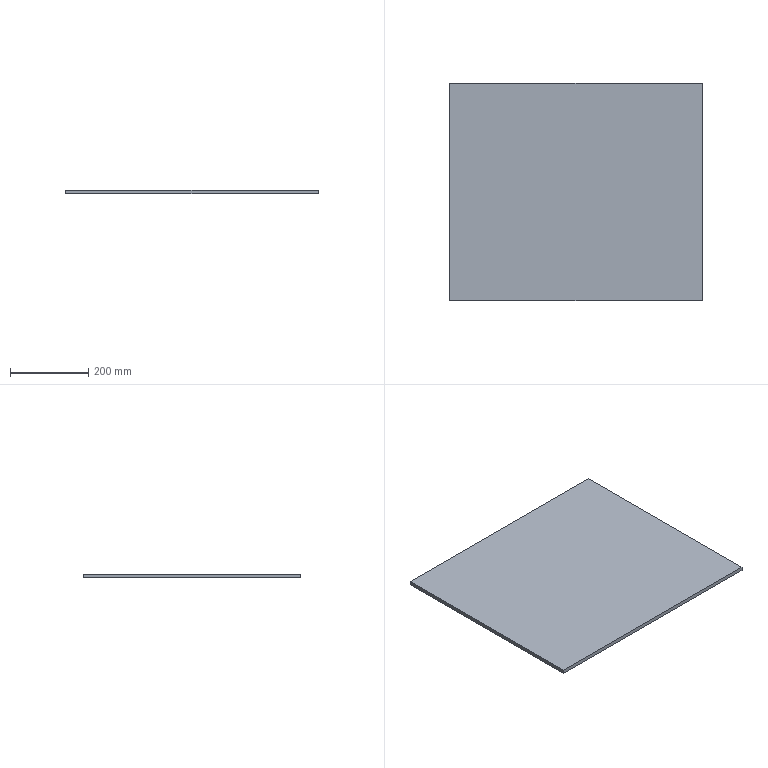Part | SolidWorks | features BaseBody 1, ICE 1 | 1 solid | 6 faces | box 645 x 555 x 10 mm | volume 3579750 mm3 | plane 6
STEP:
#1=CARTESIAN_POINT('',(115.,45.,315.));
#2=VERTEX_POINT('',#1);
#3=CARTESIAN_POINT('',(115.,45.,325.));
#4=VERTEX_POINT('',#3);
#5=CARTESIAN_POINT('',(115.,45.,315.));
#6=DIRECTION('',(0.,0.,1.));
#7=VECTOR('',#6,1000.);
#8=LINE('',#5,#7);
#9=EDGE_CURVE('',#2,#4,#8,.T.);
#10=ORIENTED_EDGE('',*,*,#9,.F.);
#11=CARTESIAN_POINT('',(760.,45.,315.));
#12=VERTEX_POINT('',#11);
#13=CARTESIAN_POINT('',(560.,45.,315.));
#14=DIRECTION('',(-1.,0.,0.));
#15=VECTOR('',#14,1000.);
#16=LINE('',#13,#15);
#17=EDGE_CURVE('',#12,#2,#16,.T.);
#18=ORIENTED_EDGE('',*,*,#17,.F.);
#19=CARTESIAN_POINT('',(760.,45.,325.));
#20=VERTEX_POINT('',#19);
#21=CARTESIAN_POINT('',(760.,45.,315.));
#22=DIRECTION('',(0.,0.,1.));
#23=VECTOR('',#22,1000.);
#24=LINE('',#21,#23);
#25=EDGE_CURVE('',#12,#20,#24,.T.);
#26=ORIENTED_EDGE('',*,*,#25,.T.);
#27=CARTESIAN_POINT('',(115.,45.,325.));
#28=DIRECTION('',(1.,0.,0.));
#29=VECTOR('',#28,1000.);
#30=LINE('',#27,#29);
#31=EDGE_CURVE('',#4,#20,#30,.T.);
#32=ORIENTED_EDGE('',*,*,#31,.F.);
#33=EDGE_LOOP('',(#10,#18,#26,#32));
#34=FACE_OUTER_BOUND('',#33,.T.);
#35=CARTESIAN_POINT('',(337.5,45.,320.));
#36=DIRECTION('',(0.,-1.,0.));
#37=DIRECTION('',(0.,0.,-1.));
#38=AXIS2_PLACEMENT_3D('',#35,#36,#37);
#39=PLANE('',#38);
#40=ADVANCED_FACE('',(#34),#39,.T.);
#41=CARTESIAN_POINT('',(115.,600.,325.));
#42=VERTEX_POINT('',#41);
#43=CARTESIAN_POINT('',(115.,600.,315.));
#44=VERTEX_POINT('',#43);
#45=CARTESIAN_POINT('',(115.,600.,325.));
#46=DIRECTION('',(0.,0.,-1.));
#47=VECTOR('',#46,1000.);
#48=LINE('',#45,#47);
#49=EDGE_CURVE('',#42,#44,#48,.T.);
#50=ORIENTED_EDGE('',*,*,#49,.F.);
#51=CARTESIAN_POINT('',(760.,600.,325.));
#52=VERTEX_POINT('',#51);
#53=CARTESIAN_POINT('',(560.,600.,325.));
#54=DIRECTION('',(-1.,0.,0.));
#55=VECTOR('',#54,1000.);
#56=LINE('',#53,#55);
#57=EDGE_CURVE('',#52,#42,#56,.T.);
#58=ORIENTED_EDGE('',*,*,#57,.F.);
#59=CARTESIAN_POINT('',(760.,600.,315.));
#60=VERTEX_POINT('',#59);
#61=CARTESIAN_POINT('',(760.,600.,315.));
#62=DIRECTION('',(0.,0.,1.));
#63=VECTOR('',#62,1000.);
#64=LINE('',#61,#63);
#65=EDGE_CURVE('',#60,#52,#64,.T.);
#66=ORIENTED_EDGE('',*,*,#65,.F.);
#67=CARTESIAN_POINT('',(115.,600.,315.));
#68=DIRECTION('',(1.,0.,0.));
#69=VECTOR('',#68,1000.);
#70=LINE('',#67,#69);
#71=EDGE_CURVE('',#44,#60,#70,.T.);
#72=ORIENTED_EDGE('',*,*,#71,.F.);
#73=EDGE_LOOP('',(#50,#58,#66,#72));
#74=FACE_OUTER_BOUND('',#73,.T.);
#75=CARTESIAN_POINT('',(337.5,600.,320.));
#76=DIRECTION('',(0.,1.,0.));
#77=DIRECTION('',(1.,0.,0.));
#78=AXIS2_PLACEMENT_3D('',#75,#76,#77);
#79=PLANE('',#78);
#80=ADVANCED_FACE('',(#74),#79,.T.);
#81=ORIENTED_EDGE('',*,*,#9,.T.);
#82=CARTESIAN_POINT('',(115.,600.,325.));
#83=DIRECTION('',(0.,-1.,0.));
#84=VECTOR('',#83,1000.);
#85=LINE('',#82,#84);
#86=EDGE_CURVE('',#42,#4,#85,.T.);
#87=ORIENTED_EDGE('',*,*,#86,.F.);
#88=ORIENTED_EDGE('',*,*,#49,.T.);
#89=CARTESIAN_POINT('',(115.,45.,315.));
#90=DIRECTION('',(0.,1.,0.));
#91=VECTOR('',#90,1000.);
#92=LINE('',#89,#91);
#93=EDGE_CURVE('',#2,#44,#92,.T.);
#94=ORIENTED_EDGE('',*,*,#93,.F.);
#95=EDGE_LOOP('',(#81,#87,#88,#94));
#96=FACE_OUTER_BOUND('',#95,.T.);
#97=CARTESIAN_POINT('',(115.,45.,315.));
#98=DIRECTION('',(-1.,0.,0.));
#99=DIRECTION('',(0.,0.,1.));
#100=AXIS2_PLACEMENT_3D('',#97,#98,#99);
#101=PLANE('',#100);
#102=ADVANCED_FACE('',(#96),#101,.T.);
#103=ORIENTED_EDGE('',*,*,#31,.T.);
#104=CARTESIAN_POINT('',(760.,600.,325.));
#105=DIRECTION('',(0.,1.,0.));
#106=VECTOR('',#105,1000.);
#107=LINE('',#104,#106);
#108=EDGE_CURVE('',#20,#52,#107,.T.);
#109=ORIENTED_EDGE('',*,*,#108,.T.);
#110=ORIENTED_EDGE('',*,*,#57,.T.);
#111=ORIENTED_EDGE('',*,*,#86,.T.);
#112=EDGE_LOOP('',(#103,#109,#110,#111));
#113=FACE_OUTER_BOUND('',#112,.T.);
#114=CARTESIAN_POINT('',(115.,45.,325.));
#115=DIRECTION('',(0.,0.,1.));
#116=DIRECTION('',(1.,0.,0.));
#117=AXIS2_PLACEMENT_3D('',#114,#115,#116);
#118=PLANE('',#117);
#119=ADVANCED_FACE('',(#113),#118,.T.);
#120=ORIENTED_EDGE('',*,*,#17,.T.);
#121=ORIENTED_EDGE('',*,*,#93,.T.);
#122=ORIENTED_EDGE('',*,*,#71,.T.);
#123=CARTESIAN_POINT('',(760.,600.,315.));
#124=DIRECTION('',(0.,1.,0.));
#125=VECTOR('',#124,1000.);
#126=LINE('',#123,#125);
#127=EDGE_CURVE('',#12,#60,#126,.T.);
#128=ORIENTED_EDGE('',*,*,#127,.F.);
#129=EDGE_LOOP('',(#120,#121,#122,#128));
#130=FACE_OUTER_BOUND('',#129,.T.);
#131=CARTESIAN_POINT('',(560.,45.,315.));
#132=DIRECTION('',(0.,0.,-1.));
#133=DIRECTION('',(0.,-1.,0.));
#134=AXIS2_PLACEMENT_3D('',#131,#132,#133);
#135=PLANE('',#134);
#136=ADVANCED_FACE('',(#130),#135,.T.);
#137=ORIENTED_EDGE('',*,*,#108,.F.);
#138=ORIENTED_EDGE('',*,*,#25,.F.);
#139=ORIENTED_EDGE('',*,*,#127,.T.);
#140=ORIENTED_EDGE('',*,*,#65,.T.);
#141=EDGE_LOOP('',(#137,#138,#139,#140));
#142=FACE_OUTER_BOUND('',#141,.T.);
#143=CARTESIAN_POINT('',(760.,600.,315.));
#144=DIRECTION('',(1.,0.,0.));
#145=DIRECTION('',(0.,1.,0.));
#146=AXIS2_PLACEMENT_3D('',#143,#144,#145);
#147=PLANE('',#146);
#148=ADVANCED_FACE('',(#142),#147,.T.);
#149=CLOSED_SHELL('',(#40,#80,#102,#119,#136,#148));
#150=MANIFOLD_SOLID_BREP('',#149);
#151=CARTESIAN_POINT('',(0.,0.,0.));
#152=DIRECTION('',(0.,0.,1.));
#153=DIRECTION('',(1.,0.,0.));
#154=AXIS2_PLACEMENT_3D('',#151,#152,#153);
#155=(LENGTH_UNIT()NAMED_UNIT(*)SI_UNIT(.MILLI.,.METRE.));
#156=UNCERTAINTY_MEASURE_WITH_UNIT(LENGTH_MEASURE(0.00001),#155,'','');
#157=(NAMED_UNIT(*)PLANE_ANGLE_UNIT()SI_UNIT($,.RADIAN.));
#158=(NAMED_UNIT(*)SI_UNIT($,.STERADIAN.)SOLID_ANGLE_UNIT());
#159=(GEOMETRIC_REPRESENTATION_CONTEXT(3)GLOBAL_UNCERTAINTY_ASSIGNED_CONTEXT((#156))GLOBAL_UNIT_ASSIGNED_CONTEXT((#155,#157,#158))REPRESENTATION_CONTEXT('',''));
#160=ADVANCED_BREP_SHAPE_REPRESENTATION('',(#150,#154),#159);